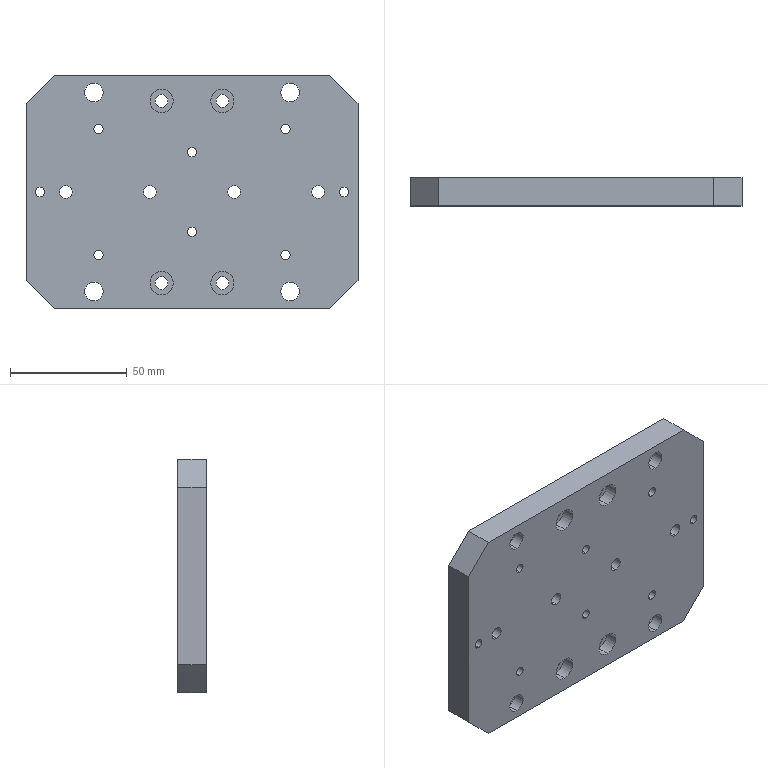Part | SolidWorks | features HoleWzd 6, Chamfer 1, Extrusion 1, ICE 1 | 1 solid | 86 faces | box 142 x 12 x 100 mm | volume 155775 mm3 | cylinder 64 | plane 22 | commonest cylinder face diameters 4 x16 5.5 x16 10 x16 8 x8 14 x8